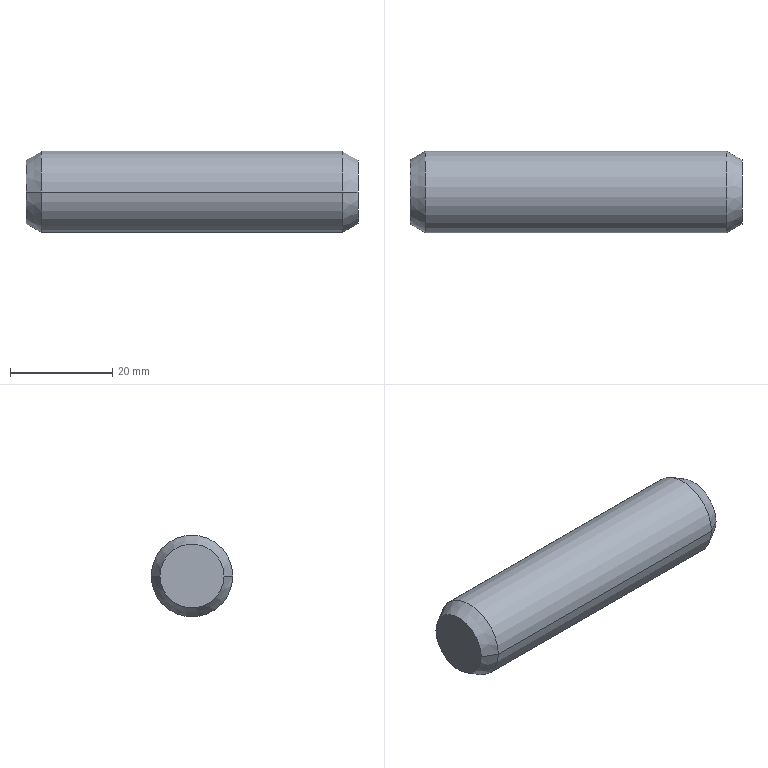Part | SolidWorks | 1 solid | 8 faces | box 65 x 16 x 16 mm | volume 12827 mm3 | cone 4 | cylinder 2 | plane 2 | commonest cylinder face diameters 16 x2
STEP:
#1=CARTESIAN_POINT('',(29.5,-8.,0.));
#2=VERTEX_POINT('',#1);
#3=CARTESIAN_POINT('',(29.5,8.,0.));
#4=VERTEX_POINT('',#3);
#5=CARTESIAN_POINT('',(29.5,0.,0.));
#6=DIRECTION('',(-1.,0.,0.));
#7=DIRECTION('',(0.,-1.,0.));
#8=AXIS2_PLACEMENT_3D('',#5,#6,#7);
#9=CIRCLE('',#8,8.);
#10=EDGE_CURVE('',#2,#4,#9,.T.);
#11=ORIENTED_EDGE('',*,*,#10,.T.);
#12=CARTESIAN_POINT('',(-29.5,8.,0.));
#13=VERTEX_POINT('',#12);
#14=CARTESIAN_POINT('',(-32.5,8.,0.));
#15=DIRECTION('',(-1.,0.,0.));
#16=VECTOR('',#15,1000.);
#17=LINE('',#14,#16);
#18=EDGE_CURVE('',#4,#13,#17,.T.);
#19=ORIENTED_EDGE('',*,*,#18,.T.);
#20=CARTESIAN_POINT('',(-29.5,-8.,0.));
#21=VERTEX_POINT('',#20);
#22=CARTESIAN_POINT('',(-29.5,0.,0.));
#23=DIRECTION('',(-1.,0.,0.));
#24=DIRECTION('',(0.,-1.,0.));
#25=AXIS2_PLACEMENT_3D('',#22,#23,#24);
#26=CIRCLE('',#25,8.);
#27=EDGE_CURVE('',#21,#13,#26,.T.);
#28=ORIENTED_EDGE('',*,*,#27,.F.);
#29=CARTESIAN_POINT('',(-32.5,-8.,0.));
#30=DIRECTION('',(-1.,0.,0.));
#31=VECTOR('',#30,1000.);
#32=LINE('',#29,#31);
#33=EDGE_CURVE('',#2,#21,#32,.T.);
#34=ORIENTED_EDGE('',*,*,#33,.F.);
#35=EDGE_LOOP('',(#11,#19,#28,#34));
#36=FACE_OUTER_BOUND('',#35,.T.);
#37=CARTESIAN_POINT('',(-32.5,0.,0.));
#38=DIRECTION('',(-1.,0.,0.));
#39=DIRECTION('',(0.,-1.,0.));
#40=AXIS2_PLACEMENT_3D('',#37,#38,#39);
#41=CYLINDRICAL_SURFACE('',#40,8.);
#42=ADVANCED_FACE('',(#36),#41,.T.);
#43=CARTESIAN_POINT('',(32.5,-6.268,0.));
#44=VERTEX_POINT('',#43);
#45=CARTESIAN_POINT('',(32.5,6.268,0.));
#46=VERTEX_POINT('',#45);
#47=CARTESIAN_POINT('',(32.5,0.,0.));
#48=DIRECTION('',(-1.,0.,0.));
#49=DIRECTION('',(0.,-1.,0.));
#50=AXIS2_PLACEMENT_3D('',#47,#48,#49);
#51=CIRCLE('',#50,6.268);
#52=EDGE_CURVE('',#44,#46,#51,.T.);
#53=ORIENTED_EDGE('',*,*,#52,.T.);
#54=CARTESIAN_POINT('',(32.5,6.268,0.));
#55=DIRECTION('',(-0.866,0.5,0.));
#56=VECTOR('',#55,1000.);
#57=LINE('',#54,#56);
#58=EDGE_CURVE('',#46,#4,#57,.T.);
#59=ORIENTED_EDGE('',*,*,#58,.T.);
#60=ORIENTED_EDGE('',*,*,#10,.F.);
#61=CARTESIAN_POINT('',(32.5,-6.268,0.));
#62=DIRECTION('',(-0.866,-0.5,0.));
#63=VECTOR('',#62,1000.);
#64=LINE('',#61,#63);
#65=EDGE_CURVE('',#44,#2,#64,.T.);
#66=ORIENTED_EDGE('',*,*,#65,.F.);
#67=EDGE_LOOP('',(#53,#59,#60,#66));
#68=FACE_OUTER_BOUND('',#67,.T.);
#69=CARTESIAN_POINT('',(32.5,0.,0.));
#70=DIRECTION('',(-1.,0.,0.));
#71=DIRECTION('',(0.,-1.,0.));
#72=AXIS2_PLACEMENT_3D('',#69,#70,#71);
#73=CONICAL_SURFACE('',#72,6.268,0.5236);
#74=ADVANCED_FACE('',(#68),#73,.T.);
#75=CARTESIAN_POINT('',(-32.5,-6.268,0.));
#76=VERTEX_POINT('',#75);
#77=CARTESIAN_POINT('',(-32.5,6.268,0.));
#78=VERTEX_POINT('',#77);
#79=CARTESIAN_POINT('',(-32.5,0.,0.));
#80=DIRECTION('',(-1.,0.,0.));
#81=DIRECTION('',(0.,-1.,0.));
#82=AXIS2_PLACEMENT_3D('',#79,#80,#81);
#83=CIRCLE('',#82,6.268);
#84=EDGE_CURVE('',#76,#78,#83,.T.);
#85=ORIENTED_EDGE('',*,*,#84,.F.);
#86=CARTESIAN_POINT('',(-29.5,-8.,0.));
#87=DIRECTION('',(0.866,-0.5,0.));
#88=VECTOR('',#87,1000.);
#89=LINE('',#86,#88);
#90=EDGE_CURVE('',#76,#21,#89,.T.);
#91=ORIENTED_EDGE('',*,*,#90,.T.);
#92=ORIENTED_EDGE('',*,*,#27,.T.);
#93=CARTESIAN_POINT('',(-29.5,8.,0.));
#94=DIRECTION('',(0.866,0.5,0.));
#95=VECTOR('',#94,1000.);
#96=LINE('',#93,#95);
#97=EDGE_CURVE('',#78,#13,#96,.T.);
#98=ORIENTED_EDGE('',*,*,#97,.F.);
#99=EDGE_LOOP('',(#85,#91,#92,#98));
#100=FACE_OUTER_BOUND('',#99,.T.);
#101=CARTESIAN_POINT('',(-29.5,0.,0.));
#102=DIRECTION('',(1.,0.,0.));
#103=DIRECTION('',(0.,1.,0.));
#104=AXIS2_PLACEMENT_3D('',#101,#102,#103);
#105=CONICAL_SURFACE('',#104,8.,0.5236);
#106=ADVANCED_FACE('',(#100),#105,.T.);
#107=ORIENTED_EDGE('',*,*,#90,.F.);
#108=CARTESIAN_POINT('',(-32.5,0.,0.));
#109=DIRECTION('',(-1.,0.,0.));
#110=DIRECTION('',(0.,-1.,0.));
#111=AXIS2_PLACEMENT_3D('',#108,#109,#110);
#112=CIRCLE('',#111,6.268);
#113=EDGE_CURVE('',#78,#76,#112,.T.);
#114=ORIENTED_EDGE('',*,*,#113,.F.);
#115=ORIENTED_EDGE('',*,*,#97,.T.);
#116=CARTESIAN_POINT('',(-29.5,0.,0.));
#117=DIRECTION('',(-1.,0.,0.));
#118=DIRECTION('',(0.,-1.,0.));
#119=AXIS2_PLACEMENT_3D('',#116,#117,#118);
#120=CIRCLE('',#119,8.);
#121=EDGE_CURVE('',#13,#21,#120,.T.);
#122=ORIENTED_EDGE('',*,*,#121,.T.);
#123=EDGE_LOOP('',(#107,#114,#115,#122));
#124=FACE_OUTER_BOUND('',#123,.T.);
#125=CARTESIAN_POINT('',(-29.5,0.,0.));
#126=DIRECTION('',(1.,0.,0.));
#127=DIRECTION('',(0.,1.,0.));
#128=AXIS2_PLACEMENT_3D('',#125,#126,#127);
#129=CONICAL_SURFACE('',#128,8.,0.5236);
#130=ADVANCED_FACE('',(#124),#129,.T.);
#131=ORIENTED_EDGE('',*,*,#113,.T.);
#132=ORIENTED_EDGE('',*,*,#84,.T.);
#133=EDGE_LOOP('',(#131,#132));
#134=FACE_OUTER_BOUND('',#133,.T.);
#135=CARTESIAN_POINT('',(-32.5,6.268,0.));
#136=DIRECTION('',(1.,0.,0.));
#137=DIRECTION('',(0.,1.,0.));
#138=AXIS2_PLACEMENT_3D('',#135,#136,#137);
#139=PLANE('',#138);
#140=ADVANCED_FACE('',(#134),#139,.F.);
#141=ORIENTED_EDGE('',*,*,#52,.F.);
#142=CARTESIAN_POINT('',(32.5,0.,0.));
#143=DIRECTION('',(-1.,0.,0.));
#144=DIRECTION('',(0.,-1.,0.));
#145=AXIS2_PLACEMENT_3D('',#142,#143,#144);
#146=CIRCLE('',#145,6.268);
#147=EDGE_CURVE('',#46,#44,#146,.T.);
#148=ORIENTED_EDGE('',*,*,#147,.F.);
#149=EDGE_LOOP('',(#141,#148));
#150=FACE_OUTER_BOUND('',#149,.T.);
#151=CARTESIAN_POINT('',(32.5,6.268,0.));
#152=DIRECTION('',(-1.,0.,0.));
#153=DIRECTION('',(0.,-1.,0.));
#154=AXIS2_PLACEMENT_3D('',#151,#152,#153);
#155=PLANE('',#154);
#156=ADVANCED_FACE('',(#150),#155,.F.);
#157=ORIENTED_EDGE('',*,*,#58,.F.);
#158=ORIENTED_EDGE('',*,*,#147,.T.);
#159=ORIENTED_EDGE('',*,*,#65,.T.);
#160=CARTESIAN_POINT('',(29.5,0.,0.));
#161=DIRECTION('',(-1.,0.,0.));
#162=DIRECTION('',(0.,-1.,0.));
#163=AXIS2_PLACEMENT_3D('',#160,#161,#162);
#164=CIRCLE('',#163,8.);
#165=EDGE_CURVE('',#4,#2,#164,.T.);
#166=ORIENTED_EDGE('',*,*,#165,.F.);
#167=EDGE_LOOP('',(#157,#158,#159,#166));
#168=FACE_OUTER_BOUND('',#167,.T.);
#169=CARTESIAN_POINT('',(32.5,0.,0.));
#170=DIRECTION('',(-1.,0.,0.));
#171=DIRECTION('',(0.,-1.,0.));
#172=AXIS2_PLACEMENT_3D('',#169,#170,#171);
#173=CONICAL_SURFACE('',#172,6.268,0.5236);
#174=ADVANCED_FACE('',(#168),#173,.T.);
#175=ORIENTED_EDGE('',*,*,#18,.F.);
#176=ORIENTED_EDGE('',*,*,#165,.T.);
#177=ORIENTED_EDGE('',*,*,#33,.T.);
#178=ORIENTED_EDGE('',*,*,#121,.F.);
#179=EDGE_LOOP('',(#175,#176,#177,#178));
#180=FACE_OUTER_BOUND('',#179,.T.);
#181=CARTESIAN_POINT('',(-32.5,0.,0.));
#182=DIRECTION('',(-1.,0.,0.));
#183=DIRECTION('',(0.,-1.,0.));
#184=AXIS2_PLACEMENT_3D('',#181,#182,#183);
#185=CYLINDRICAL_SURFACE('',#184,8.);
#186=ADVANCED_FACE('',(#180),#185,.T.);
#187=CLOSED_SHELL('',(#42,#74,#106,#130,#140,#156,#174,#186));
#188=MANIFOLD_SOLID_BREP('',#187);
#189=CARTESIAN_POINT('',(0.,0.,0.));
#190=DIRECTION('',(0.,0.,1.));
#191=DIRECTION('',(1.,0.,0.));
#192=AXIS2_PLACEMENT_3D('',#189,#190,#191);
#193=(LENGTH_UNIT()NAMED_UNIT(*)SI_UNIT(.MILLI.,.METRE.));
#194=UNCERTAINTY_MEASURE_WITH_UNIT(LENGTH_MEASURE(0.00001),#193,'','');
#195=(NAMED_UNIT(*)PLANE_ANGLE_UNIT()SI_UNIT($,.RADIAN.));
#196=(NAMED_UNIT(*)SI_UNIT($,.STERADIAN.)SOLID_ANGLE_UNIT());
#197=(GEOMETRIC_REPRESENTATION_CONTEXT(3)GLOBAL_UNCERTAINTY_ASSIGNED_CONTEXT((#194))GLOBAL_UNIT_ASSIGNED_CONTEXT((#193,#195,#196))REPRESENTATION_CONTEXT('',''));
#198=ADVANCED_BREP_SHAPE_REPRESENTATION('',(#188,#192),#197);